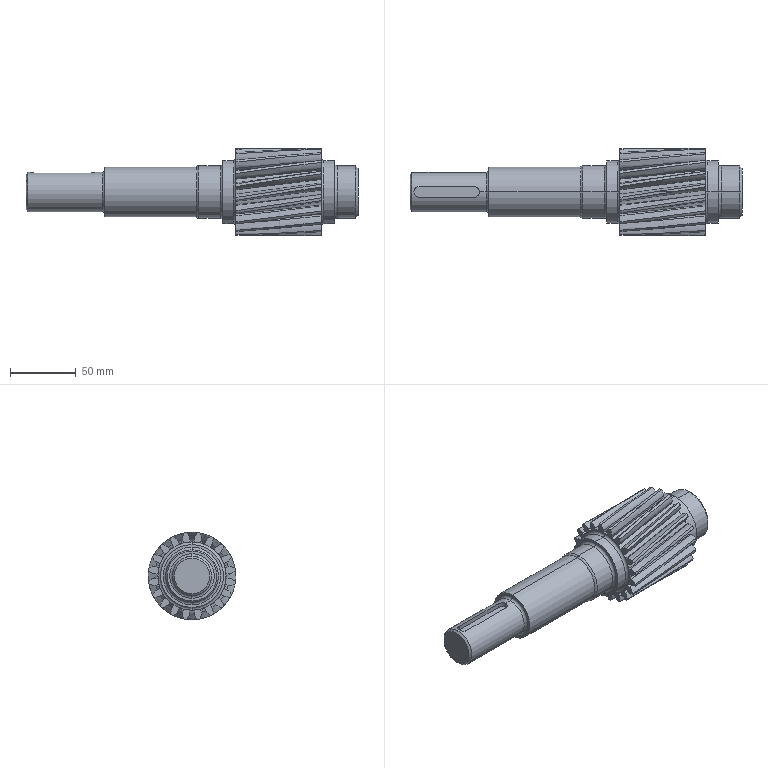Part | SolidWorks | features ICE 4, Chamfer 2, CirPattern 1, Extrusion 1, Fillet 1, Helix 1, Revolution 1, SweepCut 1 | 1 solid | 162 faces | box 253 x 66.606 x 66.606 mm | volume 387584 mm3 | spline 100 | cylinder 36 | torus 12 | plane 10 | cone 4 | commonest cylinder face diameters 66.606 x21 40 x4 48 x4 8 x3 30 x2 38 x2